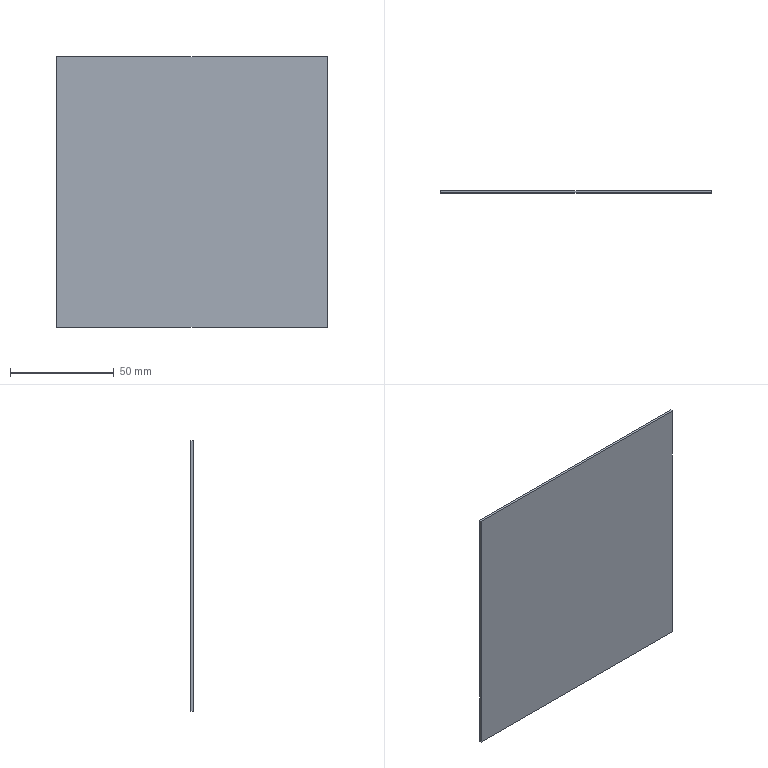Part | SolidWorks | features BaseBody 1 | 1 solid | 6 faces | box 130 x 1 x 130 mm | volume 16900 mm3 | plane 6
STEP:
#1=CARTESIAN_POINT('',(-7.753,371.5,-296.043));
#2=VERTEX_POINT('',#1);
#3=CARTESIAN_POINT('',(122.247,371.5,-296.043));
#4=VERTEX_POINT('',#3);
#5=CARTESIAN_POINT('',(57.247,371.5,-296.043));
#6=DIRECTION('',(1.,0.,0.));
#7=VECTOR('',#6,1000.);
#8=LINE('',#5,#7);
#9=EDGE_CURVE('',#2,#4,#8,.T.);
#10=ORIENTED_EDGE('',*,*,#9,.T.);
#11=CARTESIAN_POINT('',(122.247,371.5,-166.043));
#12=VERTEX_POINT('',#11);
#13=CARTESIAN_POINT('',(122.247,371.5,-276.043));
#14=DIRECTION('',(0.,0.,1.));
#15=VECTOR('',#14,1000.);
#16=LINE('',#13,#15);
#17=EDGE_CURVE('',#4,#12,#16,.T.);
#18=ORIENTED_EDGE('',*,*,#17,.T.);
#19=CARTESIAN_POINT('',(-7.753,371.5,-166.043));
#20=VERTEX_POINT('',#19);
#21=CARTESIAN_POINT('',(57.247,371.5,-166.043));
#22=DIRECTION('',(-1.,0.,0.));
#23=VECTOR('',#22,1000.);
#24=LINE('',#21,#23);
#25=EDGE_CURVE('',#12,#20,#24,.T.);
#26=ORIENTED_EDGE('',*,*,#25,.T.);
#27=CARTESIAN_POINT('',(-7.753,371.5,-276.043));
#28=DIRECTION('',(0.,0.,-1.));
#29=VECTOR('',#28,1000.);
#30=LINE('',#27,#29);
#31=EDGE_CURVE('',#20,#2,#30,.T.);
#32=ORIENTED_EDGE('',*,*,#31,.T.);
#33=EDGE_LOOP('',(#10,#18,#26,#32));
#34=FACE_OUTER_BOUND('',#33,.T.);
#35=CARTESIAN_POINT('',(57.247,371.5,-276.043));
#36=DIRECTION('',(0.,-1.,0.));
#37=DIRECTION('',(0.,0.,-1.));
#38=AXIS2_PLACEMENT_3D('',#35,#36,#37);
#39=PLANE('',#38);
#40=ADVANCED_FACE('',(#34),#39,.T.);
#41=ORIENTED_EDGE('',*,*,#17,.F.);
#42=CARTESIAN_POINT('',(122.247,372.5,-296.043));
#43=VERTEX_POINT('',#42);
#44=CARTESIAN_POINT('',(122.247,372.,-296.043));
#45=DIRECTION('',(0.,1.,0.));
#46=VECTOR('',#45,1000.);
#47=LINE('',#44,#46);
#48=EDGE_CURVE('',#4,#43,#47,.T.);
#49=ORIENTED_EDGE('',*,*,#48,.T.);
#50=CARTESIAN_POINT('',(122.247,372.5,-166.043));
#51=VERTEX_POINT('',#50);
#52=CARTESIAN_POINT('',(122.247,372.5,-276.043));
#53=DIRECTION('',(0.,0.,1.));
#54=VECTOR('',#53,1000.);
#55=LINE('',#52,#54);
#56=EDGE_CURVE('',#43,#51,#55,.T.);
#57=ORIENTED_EDGE('',*,*,#56,.T.);
#58=CARTESIAN_POINT('',(122.247,372.,-166.043));
#59=DIRECTION('',(0.,-1.,0.));
#60=VECTOR('',#59,1000.);
#61=LINE('',#58,#60);
#62=EDGE_CURVE('',#51,#12,#61,.T.);
#63=ORIENTED_EDGE('',*,*,#62,.T.);
#64=EDGE_LOOP('',(#41,#49,#57,#63));
#65=FACE_OUTER_BOUND('',#64,.T.);
#66=CARTESIAN_POINT('',(122.247,372.,-276.043));
#67=DIRECTION('',(1.,0.,0.));
#68=DIRECTION('',(0.,0.,-1.));
#69=AXIS2_PLACEMENT_3D('',#66,#67,#68);
#70=PLANE('',#69);
#71=ADVANCED_FACE('',(#65),#70,.T.);
#72=CARTESIAN_POINT('',(-7.753,372.5,-296.043));
#73=VERTEX_POINT('',#72);
#74=CARTESIAN_POINT('',(57.247,372.5,-296.043));
#75=DIRECTION('',(1.,0.,0.));
#76=VECTOR('',#75,1000.);
#77=LINE('',#74,#76);
#78=EDGE_CURVE('',#73,#43,#77,.T.);
#79=ORIENTED_EDGE('',*,*,#78,.T.);
#80=ORIENTED_EDGE('',*,*,#48,.F.);
#81=ORIENTED_EDGE('',*,*,#9,.F.);
#82=CARTESIAN_POINT('',(-7.753,372.,-296.043));
#83=DIRECTION('',(0.,1.,0.));
#84=VECTOR('',#83,1000.);
#85=LINE('',#82,#84);
#86=EDGE_CURVE('',#2,#73,#85,.T.);
#87=ORIENTED_EDGE('',*,*,#86,.T.);
#88=EDGE_LOOP('',(#79,#80,#81,#87));
#89=FACE_OUTER_BOUND('',#88,.T.);
#90=CARTESIAN_POINT('',(57.247,372.,-296.043));
#91=DIRECTION('',(0.,0.,-1.));
#92=DIRECTION('',(-1.,0.,0.));
#93=AXIS2_PLACEMENT_3D('',#90,#91,#92);
#94=PLANE('',#93);
#95=ADVANCED_FACE('',(#89),#94,.T.);
#96=ORIENTED_EDGE('',*,*,#86,.F.);
#97=ORIENTED_EDGE('',*,*,#31,.F.);
#98=CARTESIAN_POINT('',(-7.753,372.5,-166.043));
#99=VERTEX_POINT('',#98);
#100=CARTESIAN_POINT('',(-7.753,372.,-166.043));
#101=DIRECTION('',(0.,1.,0.));
#102=VECTOR('',#101,1000.);
#103=LINE('',#100,#102);
#104=EDGE_CURVE('',#20,#99,#103,.T.);
#105=ORIENTED_EDGE('',*,*,#104,.T.);
#106=CARTESIAN_POINT('',(-7.753,372.5,-276.043));
#107=DIRECTION('',(0.,0.,-1.));
#108=VECTOR('',#107,1000.);
#109=LINE('',#106,#108);
#110=EDGE_CURVE('',#99,#73,#109,.T.);
#111=ORIENTED_EDGE('',*,*,#110,.T.);
#112=EDGE_LOOP('',(#96,#97,#105,#111));
#113=FACE_OUTER_BOUND('',#112,.T.);
#114=CARTESIAN_POINT('',(-7.753,372.,-276.043));
#115=DIRECTION('',(-1.,0.,0.));
#116=DIRECTION('',(0.,0.,1.));
#117=AXIS2_PLACEMENT_3D('',#114,#115,#116);
#118=PLANE('',#117);
#119=ADVANCED_FACE('',(#113),#118,.T.);
#120=ORIENTED_EDGE('',*,*,#104,.F.);
#121=ORIENTED_EDGE('',*,*,#25,.F.);
#122=ORIENTED_EDGE('',*,*,#62,.F.);
#123=CARTESIAN_POINT('',(57.247,372.5,-166.043));
#124=DIRECTION('',(-1.,0.,0.));
#125=VECTOR('',#124,1000.);
#126=LINE('',#123,#125);
#127=EDGE_CURVE('',#51,#99,#126,.T.);
#128=ORIENTED_EDGE('',*,*,#127,.T.);
#129=EDGE_LOOP('',(#120,#121,#122,#128));
#130=FACE_OUTER_BOUND('',#129,.T.);
#131=CARTESIAN_POINT('',(57.247,372.,-166.043));
#132=DIRECTION('',(0.,0.,1.));
#133=DIRECTION('',(1.,0.,0.));
#134=AXIS2_PLACEMENT_3D('',#131,#132,#133);
#135=PLANE('',#134);
#136=ADVANCED_FACE('',(#130),#135,.T.);
#137=ORIENTED_EDGE('',*,*,#78,.F.);
#138=ORIENTED_EDGE('',*,*,#110,.F.);
#139=ORIENTED_EDGE('',*,*,#127,.F.);
#140=ORIENTED_EDGE('',*,*,#56,.F.);
#141=EDGE_LOOP('',(#137,#138,#139,#140));
#142=FACE_OUTER_BOUND('',#141,.T.);
#143=CARTESIAN_POINT('',(57.247,372.5,-276.043));
#144=DIRECTION('',(0.,1.,0.));
#145=DIRECTION('',(0.,0.,1.));
#146=AXIS2_PLACEMENT_3D('',#143,#144,#145);
#147=PLANE('',#146);
#148=ADVANCED_FACE('',(#142),#147,.T.);
#149=CLOSED_SHELL('',(#40,#71,#95,#119,#136,#148));
#150=MANIFOLD_SOLID_BREP('',#149);
#151=CARTESIAN_POINT('',(0.,0.,0.));
#152=DIRECTION('',(0.,0.,1.));
#153=DIRECTION('',(1.,0.,0.));
#154=AXIS2_PLACEMENT_3D('',#151,#152,#153);
#155=(LENGTH_UNIT()NAMED_UNIT(*)SI_UNIT(.MILLI.,.METRE.));
#156=UNCERTAINTY_MEASURE_WITH_UNIT(LENGTH_MEASURE(0.00001),#155,'','');
#157=(NAMED_UNIT(*)PLANE_ANGLE_UNIT()SI_UNIT($,.RADIAN.));
#158=(NAMED_UNIT(*)SI_UNIT($,.STERADIAN.)SOLID_ANGLE_UNIT());
#159=(GEOMETRIC_REPRESENTATION_CONTEXT(3)GLOBAL_UNCERTAINTY_ASSIGNED_CONTEXT((#156))GLOBAL_UNIT_ASSIGNED_CONTEXT((#155,#157,#158))REPRESENTATION_CONTEXT('',''));
#160=ADVANCED_BREP_SHAPE_REPRESENTATION('',(#150,#154),#159);